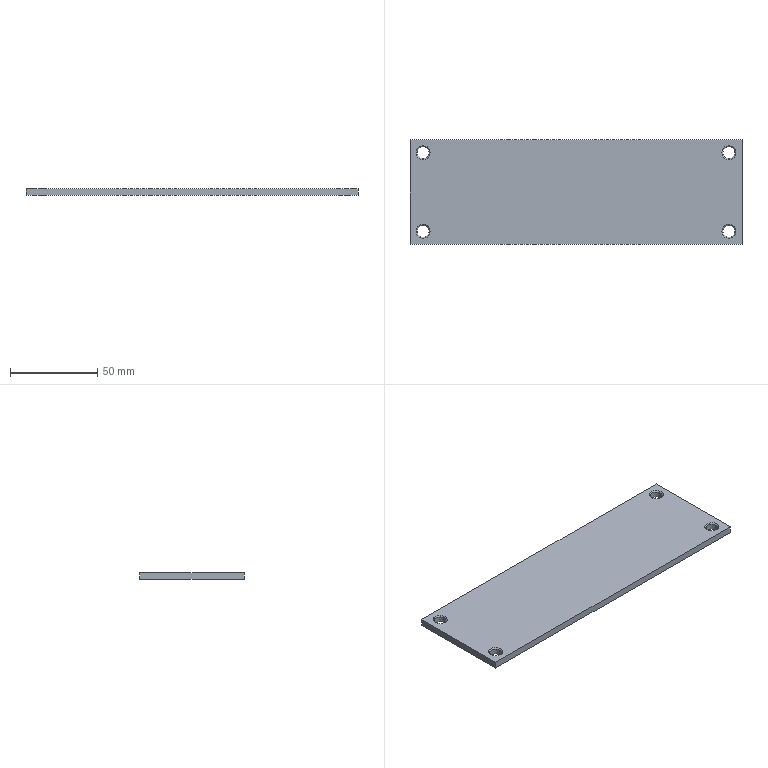Part | STEP file | Plate 2 | 1 solid | 22 faces | box 190 x 60 x 4 mm | volume 45001 mm3 | cone 8 | cylinder 8 | plane 6 | commonest cylinder face diameters 6.8 x8
STEP:
#1=CARTESIAN_POINT('',(-90.9,22.5,3.375));
#2=VERTEX_POINT('',#1);
#3=CARTESIAN_POINT('',(-84.1,22.5,3.375));
#4=VERTEX_POINT('',#3);
#5=CARTESIAN_POINT('',(-87.5,22.5,3.375));
#6=DIRECTION('',(0.,0.,1.));
#7=DIRECTION('',(1.,0.,0.));
#8=AXIS2_PLACEMENT_3D('',#5,#6,#7);
#9=CIRCLE('',#8,3.4);
#10=EDGE_CURVE('',#2,#4,#9,.T.);
#11=ORIENTED_EDGE('',*,*,#10,.F.);
#12=CARTESIAN_POINT('',(-91.525,22.5,4.));
#13=VERTEX_POINT('',#12);
#14=CARTESIAN_POINT('',(-91.525,22.5,4.));
#15=DIRECTION('',(-0.7071,0.,0.7071));
#16=VECTOR('',#15,1000.);
#17=LINE('',#14,#16);
#18=EDGE_CURVE('',#2,#13,#17,.T.);
#19=ORIENTED_EDGE('',*,*,#18,.T.);
#20=CARTESIAN_POINT('',(-83.475,22.5,4.));
#21=VERTEX_POINT('',#20);
#22=CARTESIAN_POINT('',(-87.5,22.5,4.));
#23=DIRECTION('',(0.,0.,1.));
#24=DIRECTION('',(1.,0.,0.));
#25=AXIS2_PLACEMENT_3D('',#22,#23,#24);
#26=CIRCLE('',#25,4.025);
#27=EDGE_CURVE('',#13,#21,#26,.T.);
#28=ORIENTED_EDGE('',*,*,#27,.T.);
#29=CARTESIAN_POINT('',(-83.475,22.5,4.));
#30=DIRECTION('',(0.7071,0.,0.7071));
#31=VECTOR('',#30,1000.);
#32=LINE('',#29,#31);
#33=EDGE_CURVE('',#4,#21,#32,.T.);
#34=ORIENTED_EDGE('',*,*,#33,.F.);
#35=EDGE_LOOP('',(#11,#19,#28,#34));
#36=FACE_OUTER_BOUND('',#35,.T.);
#37=CARTESIAN_POINT('',(-87.5,22.5,4.));
#38=DIRECTION('',(0.,0.,1.));
#39=DIRECTION('',(1.,0.,0.));
#40=AXIS2_PLACEMENT_3D('',#37,#38,#39);
#41=CONICAL_SURFACE('',#40,4.025,0.7854);
#42=ADVANCED_FACE('',(#36),#41,.F.);
#43=CARTESIAN_POINT('',(-84.1,22.5,0.));
#44=VERTEX_POINT('',#43);
#45=CARTESIAN_POINT('',(-90.9,22.5,0.));
#46=VERTEX_POINT('',#45);
#47=CARTESIAN_POINT('',(-87.5,22.5,0.));
#48=DIRECTION('',(0.,0.,-1.));
#49=DIRECTION('',(-1.,0.,0.));
#50=AXIS2_PLACEMENT_3D('',#47,#48,#49);
#51=CIRCLE('',#50,3.4);
#52=EDGE_CURVE('',#44,#46,#51,.T.);
#53=ORIENTED_EDGE('',*,*,#52,.T.);
#54=CARTESIAN_POINT('',(-90.9,22.5,4.));
#55=DIRECTION('',(0.,0.,1.));
#56=VECTOR('',#55,1000.);
#57=LINE('',#54,#56);
#58=EDGE_CURVE('',#46,#2,#57,.T.);
#59=ORIENTED_EDGE('',*,*,#58,.T.);
#60=ORIENTED_EDGE('',*,*,#10,.T.);
#61=CARTESIAN_POINT('',(-84.1,22.5,4.));
#62=DIRECTION('',(0.,0.,1.));
#63=VECTOR('',#62,1000.);
#64=LINE('',#61,#63);
#65=EDGE_CURVE('',#44,#4,#64,.T.);
#66=ORIENTED_EDGE('',*,*,#65,.F.);
#67=EDGE_LOOP('',(#53,#59,#60,#66));
#68=FACE_OUTER_BOUND('',#67,.T.);
#69=CARTESIAN_POINT('',(-87.5,22.5,4.));
#70=DIRECTION('',(0.,0.,1.));
#71=DIRECTION('',(1.,0.,0.));
#72=AXIS2_PLACEMENT_3D('',#69,#70,#71);
#73=CYLINDRICAL_SURFACE('',#72,3.4);
#74=ADVANCED_FACE('',(#68),#73,.F.);
#75=CARTESIAN_POINT('',(84.1,-22.5,3.375));
#76=VERTEX_POINT('',#75);
#77=CARTESIAN_POINT('',(90.9,-22.5,3.375));
#78=VERTEX_POINT('',#77);
#79=CARTESIAN_POINT('',(87.5,-22.5,3.375));
#80=DIRECTION('',(0.,0.,1.));
#81=DIRECTION('',(1.,0.,0.));
#82=AXIS2_PLACEMENT_3D('',#79,#80,#81);
#83=CIRCLE('',#82,3.4);
#84=EDGE_CURVE('',#76,#78,#83,.T.);
#85=ORIENTED_EDGE('',*,*,#84,.F.);
#86=CARTESIAN_POINT('',(83.475,-22.5,4.));
#87=VERTEX_POINT('',#86);
#88=CARTESIAN_POINT('',(83.475,-22.5,4.));
#89=DIRECTION('',(-0.7071,0.,0.7071));
#90=VECTOR('',#89,1000.);
#91=LINE('',#88,#90);
#92=EDGE_CURVE('',#76,#87,#91,.T.);
#93=ORIENTED_EDGE('',*,*,#92,.T.);
#94=CARTESIAN_POINT('',(91.525,-22.5,4.));
#95=VERTEX_POINT('',#94);
#96=CARTESIAN_POINT('',(87.5,-22.5,4.));
#97=DIRECTION('',(0.,0.,1.));
#98=DIRECTION('',(1.,0.,0.));
#99=AXIS2_PLACEMENT_3D('',#96,#97,#98);
#100=CIRCLE('',#99,4.025);
#101=EDGE_CURVE('',#87,#95,#100,.T.);
#102=ORIENTED_EDGE('',*,*,#101,.T.);
#103=CARTESIAN_POINT('',(91.525,-22.5,4.));
#104=DIRECTION('',(0.7071,0.,0.7071));
#105=VECTOR('',#104,1000.);
#106=LINE('',#103,#105);
#107=EDGE_CURVE('',#78,#95,#106,.T.);
#108=ORIENTED_EDGE('',*,*,#107,.F.);
#109=EDGE_LOOP('',(#85,#93,#102,#108));
#110=FACE_OUTER_BOUND('',#109,.T.);
#111=CARTESIAN_POINT('',(87.5,-22.5,4.));
#112=DIRECTION('',(0.,0.,1.));
#113=DIRECTION('',(1.,0.,0.));
#114=AXIS2_PLACEMENT_3D('',#111,#112,#113);
#115=CONICAL_SURFACE('',#114,4.025,0.7854);
#116=ADVANCED_FACE('',(#110),#115,.F.);
#117=CARTESIAN_POINT('',(90.9,-22.5,0.));
#118=VERTEX_POINT('',#117);
#119=CARTESIAN_POINT('',(84.1,-22.5,0.));
#120=VERTEX_POINT('',#119);
#121=CARTESIAN_POINT('',(87.5,-22.5,0.));
#122=DIRECTION('',(0.,0.,-1.));
#123=DIRECTION('',(-1.,0.,0.));
#124=AXIS2_PLACEMENT_3D('',#121,#122,#123);
#125=CIRCLE('',#124,3.4);
#126=EDGE_CURVE('',#118,#120,#125,.T.);
#127=ORIENTED_EDGE('',*,*,#126,.T.);
#128=CARTESIAN_POINT('',(84.1,-22.5,4.));
#129=DIRECTION('',(0.,0.,1.));
#130=VECTOR('',#129,1000.);
#131=LINE('',#128,#130);
#132=EDGE_CURVE('',#120,#76,#131,.T.);
#133=ORIENTED_EDGE('',*,*,#132,.T.);
#134=ORIENTED_EDGE('',*,*,#84,.T.);
#135=CARTESIAN_POINT('',(90.9,-22.5,4.));
#136=DIRECTION('',(0.,0.,1.));
#137=VECTOR('',#136,1000.);
#138=LINE('',#135,#137);
#139=EDGE_CURVE('',#118,#78,#138,.T.);
#140=ORIENTED_EDGE('',*,*,#139,.F.);
#141=EDGE_LOOP('',(#127,#133,#134,#140));
#142=FACE_OUTER_BOUND('',#141,.T.);
#143=CARTESIAN_POINT('',(87.5,-22.5,4.));
#144=DIRECTION('',(0.,0.,1.));
#145=DIRECTION('',(1.,0.,0.));
#146=AXIS2_PLACEMENT_3D('',#143,#144,#145);
#147=CYLINDRICAL_SURFACE('',#146,3.4);
#148=ADVANCED_FACE('',(#142),#147,.F.);
#149=CARTESIAN_POINT('',(84.1,22.5,3.375));
#150=VERTEX_POINT('',#149);
#151=CARTESIAN_POINT('',(90.9,22.5,3.375));
#152=VERTEX_POINT('',#151);
#153=CARTESIAN_POINT('',(87.5,22.5,3.375));
#154=DIRECTION('',(0.,0.,1.));
#155=DIRECTION('',(1.,0.,0.));
#156=AXIS2_PLACEMENT_3D('',#153,#154,#155);
#157=CIRCLE('',#156,3.4);
#158=EDGE_CURVE('',#150,#152,#157,.T.);
#159=ORIENTED_EDGE('',*,*,#158,.F.);
#160=CARTESIAN_POINT('',(83.475,22.5,4.));
#161=VERTEX_POINT('',#160);
#162=CARTESIAN_POINT('',(83.475,22.5,4.));
#163=DIRECTION('',(-0.7071,0.,0.7071));
#164=VECTOR('',#163,1000.);
#165=LINE('',#162,#164);
#166=EDGE_CURVE('',#150,#161,#165,.T.);
#167=ORIENTED_EDGE('',*,*,#166,.T.);
#168=CARTESIAN_POINT('',(91.525,22.5,4.));
#169=VERTEX_POINT('',#168);
#170=CARTESIAN_POINT('',(87.5,22.5,4.));
#171=DIRECTION('',(0.,0.,1.));
#172=DIRECTION('',(1.,0.,0.));
#173=AXIS2_PLACEMENT_3D('',#170,#171,#172);
#174=CIRCLE('',#173,4.025);
#175=EDGE_CURVE('',#161,#169,#174,.T.);
#176=ORIENTED_EDGE('',*,*,#175,.T.);
#177=CARTESIAN_POINT('',(91.525,22.5,4.));
#178=DIRECTION('',(0.7071,0.,0.7071));
#179=VECTOR('',#178,1000.);
#180=LINE('',#177,#179);
#181=EDGE_CURVE('',#152,#169,#180,.T.);
#182=ORIENTED_EDGE('',*,*,#181,.F.);
#183=EDGE_LOOP('',(#159,#167,#176,#182));
#184=FACE_OUTER_BOUND('',#183,.T.);
#185=CARTESIAN_POINT('',(87.5,22.5,4.));
#186=DIRECTION('',(0.,0.,1.));
#187=DIRECTION('',(1.,0.,0.));
#188=AXIS2_PLACEMENT_3D('',#185,#186,#187);
#189=CONICAL_SURFACE('',#188,4.025,0.7854);
#190=ADVANCED_FACE('',(#184),#189,.F.);
#191=CARTESIAN_POINT('',(90.9,22.5,0.));
#192=VERTEX_POINT('',#191);
#193=CARTESIAN_POINT('',(84.1,22.5,0.));
#194=VERTEX_POINT('',#193);
#195=CARTESIAN_POINT('',(87.5,22.5,0.));
#196=DIRECTION('',(0.,0.,-1.));
#197=DIRECTION('',(-1.,0.,0.));
#198=AXIS2_PLACEMENT_3D('',#195,#196,#197);
#199=CIRCLE('',#198,3.4);
#200=EDGE_CURVE('',#192,#194,#199,.T.);
#201=ORIENTED_EDGE('',*,*,#200,.T.);
#202=CARTESIAN_POINT('',(84.1,22.5,4.));
#203=DIRECTION('',(0.,0.,1.));
#204=VECTOR('',#203,1000.);
#205=LINE('',#202,#204);
#206=EDGE_CURVE('',#194,#150,#205,.T.);
#207=ORIENTED_EDGE('',*,*,#206,.T.);
#208=ORIENTED_EDGE('',*,*,#158,.T.);
#209=CARTESIAN_POINT('',(90.9,22.5,4.));
#210=DIRECTION('',(0.,0.,1.));
#211=VECTOR('',#210,1000.);
#212=LINE('',#209,#211);
#213=EDGE_CURVE('',#192,#152,#212,.T.);
#214=ORIENTED_EDGE('',*,*,#213,.F.);
#215=EDGE_LOOP('',(#201,#207,#208,#214));
#216=FACE_OUTER_BOUND('',#215,.T.);
#217=CARTESIAN_POINT('',(87.5,22.5,4.));
#218=DIRECTION('',(0.,0.,1.));
#219=DIRECTION('',(1.,0.,0.));
#220=AXIS2_PLACEMENT_3D('',#217,#218,#219);
#221=CYLINDRICAL_SURFACE('',#220,3.4);
#222=ADVANCED_FACE('',(#216),#221,.F.);
#223=CARTESIAN_POINT('',(-90.9,-22.5,3.375));
#224=VERTEX_POINT('',#223);
#225=CARTESIAN_POINT('',(-84.1,-22.5,3.375));
#226=VERTEX_POINT('',#225);
#227=CARTESIAN_POINT('',(-87.5,-22.5,3.375));
#228=DIRECTION('',(0.,0.,1.));
#229=DIRECTION('',(1.,0.,0.));
#230=AXIS2_PLACEMENT_3D('',#227,#228,#229);
#231=CIRCLE('',#230,3.4);
#232=EDGE_CURVE('',#224,#226,#231,.T.);
#233=ORIENTED_EDGE('',*,*,#232,.F.);
#234=CARTESIAN_POINT('',(-91.525,-22.5,4.));
#235=VERTEX_POINT('',#234);
#236=CARTESIAN_POINT('',(-91.525,-22.5,4.));
#237=DIRECTION('',(-0.7071,0.,0.7071));
#238=VECTOR('',#237,1000.);
#239=LINE('',#236,#238);
#240=EDGE_CURVE('',#224,#235,#239,.T.);
#241=ORIENTED_EDGE('',*,*,#240,.T.);
#242=CARTESIAN_POINT('',(-83.475,-22.5,4.));
#243=VERTEX_POINT('',#242);
#244=CARTESIAN_POINT('',(-87.5,-22.5,4.));
#245=DIRECTION('',(0.,0.,1.));
#246=DIRECTION('',(1.,0.,0.));
#247=AXIS2_PLACEMENT_3D('',#244,#245,#246);
#248=CIRCLE('',#247,4.025);
#249=EDGE_CURVE('',#235,#243,#248,.T.);
#250=ORIENTED_EDGE('',*,*,#249,.T.);
#251=CARTESIAN_POINT('',(-83.475,-22.5,4.));
#252=DIRECTION('',(0.7071,0.,0.7071));
#253=VECTOR('',#252,1000.);
#254=LINE('',#251,#253);
#255=EDGE_CURVE('',#226,#243,#254,.T.);
#256=ORIENTED_EDGE('',*,*,#255,.F.);
#257=EDGE_LOOP('',(#233,#241,#250,#256));
#258=FACE_OUTER_BOUND('',#257,.T.);
#259=CARTESIAN_POINT('',(-87.5,-22.5,4.));
#260=DIRECTION('',(0.,0.,1.));
#261=DIRECTION('',(1.,0.,0.));
#262=AXIS2_PLACEMENT_3D('',#259,#260,#261);
#263=CONICAL_SURFACE('',#262,4.025,0.7854);
#264=ADVANCED_FACE('',(#258),#263,.F.);
#265=CARTESIAN_POINT('',(-84.1,-22.5,0.));
#266=VERTEX_POINT('',#265);
#267=CARTESIAN_POINT('',(-90.9,-22.5,0.));
#268=VERTEX_POINT('',#267);
#269=CARTESIAN_POINT('',(-87.5,-22.5,0.));
#270=DIRECTION('',(0.,0.,-1.));
#271=DIRECTION('',(-1.,0.,0.));
#272=AXIS2_PLACEMENT_3D('',#269,#270,#271);
#273=CIRCLE('',#272,3.4);
#274=EDGE_CURVE('',#266,#268,#273,.T.);
#275=ORIENTED_EDGE('',*,*,#274,.T.);
#276=CARTESIAN_POINT('',(-90.9,-22.5,4.));
#277=DIRECTION('',(0.,0.,1.));
#278=VECTOR('',#277,1000.);
#279=LINE('',#276,#278);
#280=EDGE_CURVE('',#268,#224,#279,.T.);
#281=ORIENTED_EDGE('',*,*,#280,.T.);
#282=ORIENTED_EDGE('',*,*,#232,.T.);
#283=CARTESIAN_POINT('',(-84.1,-22.5,4.));
#284=DIRECTION('',(0.,0.,1.));
#285=VECTOR('',#284,1000.);
#286=LINE('',#283,#285);
#287=EDGE_CURVE('',#266,#226,#286,.T.);
#288=ORIENTED_EDGE('',*,*,#287,.F.);
#289=EDGE_LOOP('',(#275,#281,#282,#288));
#290=FACE_OUTER_BOUND('',#289,.T.);
#291=CARTESIAN_POINT('',(-87.5,-22.5,4.));
#292=DIRECTION('',(0.,0.,1.));
#293=DIRECTION('',(1.,0.,0.));
#294=AXIS2_PLACEMENT_3D('',#291,#292,#293);
#295=CYLINDRICAL_SURFACE('',#294,3.4);
#296=ADVANCED_FACE('',(#290),#295,.F.);
#297=CARTESIAN_POINT('',(95.,30.,4.));
#298=VERTEX_POINT('',#297);
#299=CARTESIAN_POINT('',(-95.,30.,4.));
#300=VERTEX_POINT('',#299);
#301=CARTESIAN_POINT('',(-95.,30.,4.));
#302=DIRECTION('',(-1.,0.,0.));
#303=VECTOR('',#302,1000.);
#304=LINE('',#301,#303);
#305=EDGE_CURVE('',#298,#300,#304,.T.);
#306=ORIENTED_EDGE('',*,*,#305,.T.);
#307=CARTESIAN_POINT('',(-95.,-30.,4.));
#308=VERTEX_POINT('',#307);
#309=CARTESIAN_POINT('',(-95.,30.001,4.));
#310=DIRECTION('',(0.,-1.,0.));
#311=VECTOR('',#310,1000.);
#312=LINE('',#309,#311);
#313=EDGE_CURVE('',#300,#308,#312,.T.);
#314=ORIENTED_EDGE('',*,*,#313,.T.);
#315=CARTESIAN_POINT('',(95.,-30.,4.));
#316=VERTEX_POINT('',#315);
#317=CARTESIAN_POINT('',(-95.,-30.,4.));
#318=DIRECTION('',(1.,0.,0.));
#319=VECTOR('',#318,1000.);
#320=LINE('',#317,#319);
#321=EDGE_CURVE('',#308,#316,#320,.T.);
#322=ORIENTED_EDGE('',*,*,#321,.T.);
#323=CARTESIAN_POINT('',(95.,-30.,4.));
#324=DIRECTION('',(0.,1.,0.));
#325=VECTOR('',#324,1000.);
#326=LINE('',#323,#325);
#327=EDGE_CURVE('',#316,#298,#326,.T.);
#328=ORIENTED_EDGE('',*,*,#327,.T.);
#329=EDGE_LOOP('',(#306,#314,#322,#328));
#330=FACE_OUTER_BOUND('',#329,.T.);
#331=CARTESIAN_POINT('',(-87.5,-22.5,4.));
#332=DIRECTION('',(0.,0.,1.));
#333=DIRECTION('',(1.,0.,0.));
#334=AXIS2_PLACEMENT_3D('',#331,#332,#333);
#335=CIRCLE('',#334,4.025);
#336=EDGE_CURVE('',#243,#235,#335,.T.);
#337=ORIENTED_EDGE('',*,*,#336,.F.);
#338=ORIENTED_EDGE('',*,*,#249,.F.);
#339=EDGE_LOOP('',(#337,#338));
#340=FACE_BOUND('',#339,.T.);
#341=CARTESIAN_POINT('',(87.5,22.5,4.));
#342=DIRECTION('',(0.,0.,1.));
#343=DIRECTION('',(1.,0.,0.));
#344=AXIS2_PLACEMENT_3D('',#341,#342,#343);
#345=CIRCLE('',#344,4.025);
#346=EDGE_CURVE('',#169,#161,#345,.T.);
#347=ORIENTED_EDGE('',*,*,#346,.F.);
#348=ORIENTED_EDGE('',*,*,#175,.F.);
#349=EDGE_LOOP('',(#347,#348));
#350=FACE_BOUND('',#349,.T.);
#351=CARTESIAN_POINT('',(87.5,-22.5,4.));
#352=DIRECTION('',(0.,0.,1.));
#353=DIRECTION('',(1.,0.,0.));
#354=AXIS2_PLACEMENT_3D('',#351,#352,#353);
#355=CIRCLE('',#354,4.025);
#356=EDGE_CURVE('',#95,#87,#355,.T.);
#357=ORIENTED_EDGE('',*,*,#356,.F.);
#358=ORIENTED_EDGE('',*,*,#101,.F.);
#359=EDGE_LOOP('',(#357,#358));
#360=FACE_BOUND('',#359,.T.);
#361=CARTESIAN_POINT('',(-87.5,22.5,4.));
#362=DIRECTION('',(0.,0.,1.));
#363=DIRECTION('',(1.,0.,0.));
#364=AXIS2_PLACEMENT_3D('',#361,#362,#363);
#365=CIRCLE('',#364,4.025);
#366=EDGE_CURVE('',#21,#13,#365,.T.);
#367=ORIENTED_EDGE('',*,*,#366,.F.);
#368=ORIENTED_EDGE('',*,*,#27,.F.);
#369=EDGE_LOOP('',(#367,#368));
#370=FACE_BOUND('',#369,.T.);
#371=CARTESIAN_POINT('',(0.,0.,4.));
#372=DIRECTION('',(0.,0.,-1.));
#373=DIRECTION('',(-1.,0.,0.));
#374=AXIS2_PLACEMENT_3D('',#371,#372,#373);
#375=PLANE('',#374);
#376=ADVANCED_FACE('',(#330,#340,#350,#360,#370),#375,.F.);
#377=CARTESIAN_POINT('',(95.,-30.,0.));
#378=VERTEX_POINT('',#377);
#379=CARTESIAN_POINT('',(95.,30.,0.));
#380=VERTEX_POINT('',#379);
#381=CARTESIAN_POINT('',(95.,-30.,0.));
#382=DIRECTION('',(0.,1.,0.));
#383=VECTOR('',#382,1000.);
#384=LINE('',#381,#383);
#385=EDGE_CURVE('',#378,#380,#384,.T.);
#386=ORIENTED_EDGE('',*,*,#385,.T.);
#387=CARTESIAN_POINT('',(95.,30.,4.));
#388=DIRECTION('',(0.,0.,-1.));
#389=VECTOR('',#388,1000.);
#390=LINE('',#387,#389);
#391=EDGE_CURVE('',#298,#380,#390,.T.);
#392=ORIENTED_EDGE('',*,*,#391,.F.);
#393=ORIENTED_EDGE('',*,*,#327,.F.);
#394=CARTESIAN_POINT('',(95.,-30.,4.));
#395=DIRECTION('',(0.,0.,-1.));
#396=VECTOR('',#395,1000.);
#397=LINE('',#394,#396);
#398=EDGE_CURVE('',#316,#378,#397,.T.);
#399=ORIENTED_EDGE('',*,*,#398,.T.);
#400=EDGE_LOOP('',(#386,#392,#393,#399));
#401=FACE_OUTER_BOUND('',#400,.T.);
#402=CARTESIAN_POINT('',(95.,-30.,4.));
#403=DIRECTION('',(-1.,0.,0.));
#404=DIRECTION('',(0.,0.,1.));
#405=AXIS2_PLACEMENT_3D('',#402,#403,#404);
#406=PLANE('',#405);
#407=ADVANCED_FACE('',(#401),#406,.F.);
#408=CARTESIAN_POINT('',(-95.,30.,0.));
#409=VERTEX_POINT('',#408);
#410=CARTESIAN_POINT('',(-95.,30.,4.));
#411=DIRECTION('',(0.,0.,-1.));
#412=VECTOR('',#411,1000.);
#413=LINE('',#410,#412);
#414=EDGE_CURVE('',#300,#409,#413,.T.);
#415=ORIENTED_EDGE('',*,*,#414,.F.);
#416=ORIENTED_EDGE('',*,*,#305,.F.);
#417=ORIENTED_EDGE('',*,*,#391,.T.);
#418=CARTESIAN_POINT('',(-95.,30.,0.));
#419=DIRECTION('',(-1.,0.,0.));
#420=VECTOR('',#419,1000.);
#421=LINE('',#418,#420);
#422=EDGE_CURVE('',#380,#409,#421,.T.);
#423=ORIENTED_EDGE('',*,*,#422,.T.);
#424=EDGE_LOOP('',(#415,#416,#417,#423));
#425=FACE_OUTER_BOUND('',#424,.T.);
#426=CARTESIAN_POINT('',(-95.,30.,4.));
#427=DIRECTION('',(0.,-1.,0.));
#428=DIRECTION('',(0.,0.,-1.));
#429=AXIS2_PLACEMENT_3D('',#426,#427,#428);
#430=PLANE('',#429);
#431=ADVANCED_FACE('',(#425),#430,.F.);
#432=CARTESIAN_POINT('',(-95.,-30.,0.));
#433=VERTEX_POINT('',#432);
#434=CARTESIAN_POINT('',(-95.,-30.,4.));
#435=DIRECTION('',(0.,0.,-1.));
#436=VECTOR('',#435,1000.);
#437=LINE('',#434,#436);
#438=EDGE_CURVE('',#308,#433,#437,.T.);
#439=ORIENTED_EDGE('',*,*,#438,.F.);
#440=ORIENTED_EDGE('',*,*,#313,.F.);
#441=ORIENTED_EDGE('',*,*,#414,.T.);
#442=CARTESIAN_POINT('',(-95.,-30.,0.));
#443=DIRECTION('',(0.,-1.,0.));
#444=VECTOR('',#443,1000.);
#445=LINE('',#442,#444);
#446=EDGE_CURVE('',#409,#433,#445,.T.);
#447=ORIENTED_EDGE('',*,*,#446,.T.);
#448=EDGE_LOOP('',(#439,#440,#441,#447));
#449=FACE_OUTER_BOUND('',#448,.T.);
#450=CARTESIAN_POINT('',(-95.,-30.,4.));
#451=DIRECTION('',(1.,0.,0.));
#452=DIRECTION('',(0.,0.,-1.));
#453=AXIS2_PLACEMENT_3D('',#450,#451,#452);
#454=PLANE('',#453);
#455=ADVANCED_FACE('',(#449),#454,.F.);
#456=ORIENTED_EDGE('',*,*,#321,.F.);
#457=ORIENTED_EDGE('',*,*,#438,.T.);
#458=CARTESIAN_POINT('',(-95.,-30.,0.));
#459=DIRECTION('',(1.,0.,0.));
#460=VECTOR('',#459,1000.);
#461=LINE('',#458,#460);
#462=EDGE_CURVE('',#433,#378,#461,.T.);
#463=ORIENTED_EDGE('',*,*,#462,.T.);
#464=ORIENTED_EDGE('',*,*,#398,.F.);
#465=EDGE_LOOP('',(#456,#457,#463,#464));
#466=FACE_OUTER_BOUND('',#465,.T.);
#467=CARTESIAN_POINT('',(-95.,-30.,4.));
#468=DIRECTION('',(0.,1.,0.));
#469=DIRECTION('',(0.,0.,1.));
#470=AXIS2_PLACEMENT_3D('',#467,#468,#469);
#471=PLANE('',#470);
#472=ADVANCED_FACE('',(#466),#471,.F.);
#473=ORIENTED_EDGE('',*,*,#52,.F.);
#474=CARTESIAN_POINT('',(-87.5,22.5,0.));
#475=DIRECTION('',(0.,0.,-1.));
#476=DIRECTION('',(-1.,0.,0.));
#477=AXIS2_PLACEMENT_3D('',#474,#475,#476);
#478=CIRCLE('',#477,3.4);
#479=EDGE_CURVE('',#46,#44,#478,.T.);
#480=ORIENTED_EDGE('',*,*,#479,.F.);
#481=EDGE_LOOP('',(#473,#480));
#482=FACE_BOUND('',#481,.T.);
#483=ORIENTED_EDGE('',*,*,#126,.F.);
#484=CARTESIAN_POINT('',(87.5,-22.5,0.));
#485=DIRECTION('',(0.,0.,-1.));
#486=DIRECTION('',(-1.,0.,0.));
#487=AXIS2_PLACEMENT_3D('',#484,#485,#486);
#488=CIRCLE('',#487,3.4);
#489=EDGE_CURVE('',#120,#118,#488,.T.);
#490=ORIENTED_EDGE('',*,*,#489,.F.);
#491=EDGE_LOOP('',(#483,#490));
#492=FACE_BOUND('',#491,.T.);
#493=ORIENTED_EDGE('',*,*,#200,.F.);
#494=CARTESIAN_POINT('',(87.5,22.5,0.));
#495=DIRECTION('',(0.,0.,-1.));
#496=DIRECTION('',(-1.,0.,0.));
#497=AXIS2_PLACEMENT_3D('',#494,#495,#496);
#498=CIRCLE('',#497,3.4);
#499=EDGE_CURVE('',#194,#192,#498,.T.);
#500=ORIENTED_EDGE('',*,*,#499,.F.);
#501=EDGE_LOOP('',(#493,#500));
#502=FACE_BOUND('',#501,.T.);
#503=ORIENTED_EDGE('',*,*,#274,.F.);
#504=CARTESIAN_POINT('',(-87.5,-22.5,0.));
#505=DIRECTION('',(0.,0.,-1.));
#506=DIRECTION('',(-1.,0.,0.));
#507=AXIS2_PLACEMENT_3D('',#504,#505,#506);
#508=CIRCLE('',#507,3.4);
#509=EDGE_CURVE('',#268,#266,#508,.T.);
#510=ORIENTED_EDGE('',*,*,#509,.F.);
#511=EDGE_LOOP('',(#503,#510));
#512=FACE_BOUND('',#511,.T.);
#513=ORIENTED_EDGE('',*,*,#385,.F.);
#514=ORIENTED_EDGE('',*,*,#462,.F.);
#515=ORIENTED_EDGE('',*,*,#446,.F.);
#516=ORIENTED_EDGE('',*,*,#422,.F.);
#517=EDGE_LOOP('',(#513,#514,#515,#516));
#518=FACE_OUTER_BOUND('',#517,.T.);
#519=CARTESIAN_POINT('',(0.,0.,0.));
#520=DIRECTION('',(0.,0.,-1.));
#521=DIRECTION('',(-1.,0.,0.));
#522=AXIS2_PLACEMENT_3D('',#519,#520,#521);
#523=PLANE('',#522);
#524=ADVANCED_FACE('',(#482,#492,#502,#512,#518),#523,.T.);
#525=ORIENTED_EDGE('',*,*,#280,.F.);
#526=ORIENTED_EDGE('',*,*,#509,.T.);
#527=ORIENTED_EDGE('',*,*,#287,.T.);
#528=CARTESIAN_POINT('',(-87.5,-22.5,3.375));
#529=DIRECTION('',(0.,0.,1.));
#530=DIRECTION('',(1.,0.,0.));
#531=AXIS2_PLACEMENT_3D('',#528,#529,#530);
#532=CIRCLE('',#531,3.4);
#533=EDGE_CURVE('',#226,#224,#532,.T.);
#534=ORIENTED_EDGE('',*,*,#533,.T.);
#535=EDGE_LOOP('',(#525,#526,#527,#534));
#536=FACE_OUTER_BOUND('',#535,.T.);
#537=CARTESIAN_POINT('',(-87.5,-22.5,4.));
#538=DIRECTION('',(0.,0.,1.));
#539=DIRECTION('',(1.,0.,0.));
#540=AXIS2_PLACEMENT_3D('',#537,#538,#539);
#541=CYLINDRICAL_SURFACE('',#540,3.4);
#542=ADVANCED_FACE('',(#536),#541,.F.);
#543=ORIENTED_EDGE('',*,*,#240,.F.);
#544=ORIENTED_EDGE('',*,*,#533,.F.);
#545=ORIENTED_EDGE('',*,*,#255,.T.);
#546=ORIENTED_EDGE('',*,*,#336,.T.);
#547=EDGE_LOOP('',(#543,#544,#545,#546));
#548=FACE_OUTER_BOUND('',#547,.T.);
#549=CARTESIAN_POINT('',(-87.5,-22.5,4.));
#550=DIRECTION('',(0.,0.,1.));
#551=DIRECTION('',(1.,0.,0.));
#552=AXIS2_PLACEMENT_3D('',#549,#550,#551);
#553=CONICAL_SURFACE('',#552,4.025,0.7854);
#554=ADVANCED_FACE('',(#548),#553,.F.);
#555=ORIENTED_EDGE('',*,*,#206,.F.);
#556=ORIENTED_EDGE('',*,*,#499,.T.);
#557=ORIENTED_EDGE('',*,*,#213,.T.);
#558=CARTESIAN_POINT('',(87.5,22.5,3.375));
#559=DIRECTION('',(0.,0.,1.));
#560=DIRECTION('',(1.,0.,0.));
#561=AXIS2_PLACEMENT_3D('',#558,#559,#560);
#562=CIRCLE('',#561,3.4);
#563=EDGE_CURVE('',#152,#150,#562,.T.);
#564=ORIENTED_EDGE('',*,*,#563,.T.);
#565=EDGE_LOOP('',(#555,#556,#557,#564));
#566=FACE_OUTER_BOUND('',#565,.T.);
#567=CARTESIAN_POINT('',(87.5,22.5,4.));
#568=DIRECTION('',(0.,0.,1.));
#569=DIRECTION('',(1.,0.,0.));
#570=AXIS2_PLACEMENT_3D('',#567,#568,#569);
#571=CYLINDRICAL_SURFACE('',#570,3.4);
#572=ADVANCED_FACE('',(#566),#571,.F.);
#573=ORIENTED_EDGE('',*,*,#166,.F.);
#574=ORIENTED_EDGE('',*,*,#563,.F.);
#575=ORIENTED_EDGE('',*,*,#181,.T.);
#576=ORIENTED_EDGE('',*,*,#346,.T.);
#577=EDGE_LOOP('',(#573,#574,#575,#576));
#578=FACE_OUTER_BOUND('',#577,.T.);
#579=CARTESIAN_POINT('',(87.5,22.5,4.));
#580=DIRECTION('',(0.,0.,1.));
#581=DIRECTION('',(1.,0.,0.));
#582=AXIS2_PLACEMENT_3D('',#579,#580,#581);
#583=CONICAL_SURFACE('',#582,4.025,0.7854);
#584=ADVANCED_FACE('',(#578),#583,.F.);
#585=ORIENTED_EDGE('',*,*,#132,.F.);
#586=ORIENTED_EDGE('',*,*,#489,.T.);
#587=ORIENTED_EDGE('',*,*,#139,.T.);
#588=CARTESIAN_POINT('',(87.5,-22.5,3.375));
#589=DIRECTION('',(0.,0.,1.));
#590=DIRECTION('',(1.,0.,0.));
#591=AXIS2_PLACEMENT_3D('',#588,#589,#590);
#592=CIRCLE('',#591,3.4);
#593=EDGE_CURVE('',#78,#76,#592,.T.);
#594=ORIENTED_EDGE('',*,*,#593,.T.);
#595=EDGE_LOOP('',(#585,#586,#587,#594));
#596=FACE_OUTER_BOUND('',#595,.T.);
#597=CARTESIAN_POINT('',(87.5,-22.5,4.));
#598=DIRECTION('',(0.,0.,1.));
#599=DIRECTION('',(1.,0.,0.));
#600=AXIS2_PLACEMENT_3D('',#597,#598,#599);
#601=CYLINDRICAL_SURFACE('',#600,3.4);
#602=ADVANCED_FACE('',(#596),#601,.F.);
#603=ORIENTED_EDGE('',*,*,#92,.F.);
#604=ORIENTED_EDGE('',*,*,#593,.F.);
#605=ORIENTED_EDGE('',*,*,#107,.T.);
#606=ORIENTED_EDGE('',*,*,#356,.T.);
#607=EDGE_LOOP('',(#603,#604,#605,#606));
#608=FACE_OUTER_BOUND('',#607,.T.);
#609=CARTESIAN_POINT('',(87.5,-22.5,4.));
#610=DIRECTION('',(0.,0.,1.));
#611=DIRECTION('',(1.,0.,0.));
#612=AXIS2_PLACEMENT_3D('',#609,#610,#611);
#613=CONICAL_SURFACE('',#612,4.025,0.7854);
#614=ADVANCED_FACE('',(#608),#613,.F.);
#615=ORIENTED_EDGE('',*,*,#58,.F.);
#616=ORIENTED_EDGE('',*,*,#479,.T.);
#617=ORIENTED_EDGE('',*,*,#65,.T.);
#618=CARTESIAN_POINT('',(-87.5,22.5,3.375));
#619=DIRECTION('',(0.,0.,1.));
#620=DIRECTION('',(1.,0.,0.));
#621=AXIS2_PLACEMENT_3D('',#618,#619,#620);
#622=CIRCLE('',#621,3.4);
#623=EDGE_CURVE('',#4,#2,#622,.T.);
#624=ORIENTED_EDGE('',*,*,#623,.T.);
#625=EDGE_LOOP('',(#615,#616,#617,#624));
#626=FACE_OUTER_BOUND('',#625,.T.);
#627=CARTESIAN_POINT('',(-87.5,22.5,4.));
#628=DIRECTION('',(0.,0.,1.));
#629=DIRECTION('',(1.,0.,0.));
#630=AXIS2_PLACEMENT_3D('',#627,#628,#629);
#631=CYLINDRICAL_SURFACE('',#630,3.4);
#632=ADVANCED_FACE('',(#626),#631,.F.);
#633=ORIENTED_EDGE('',*,*,#18,.F.);
#634=ORIENTED_EDGE('',*,*,#623,.F.);
#635=ORIENTED_EDGE('',*,*,#33,.T.);
#636=ORIENTED_EDGE('',*,*,#366,.T.);
#637=EDGE_LOOP('',(#633,#634,#635,#636));
#638=FACE_OUTER_BOUND('',#637,.T.);
#639=CARTESIAN_POINT('',(-87.5,22.5,4.));
#640=DIRECTION('',(0.,0.,1.));
#641=DIRECTION('',(1.,0.,0.));
#642=AXIS2_PLACEMENT_3D('',#639,#640,#641);
#643=CONICAL_SURFACE('',#642,4.025,0.7854);
#644=ADVANCED_FACE('',(#638),#643,.F.);
#645=CLOSED_SHELL('',(#42,#74,#116,#148,#190,#222,#264,#296,#376,#407,#431,#455,#472,#524,#542,#554,#572,#584,#602,#614,#632,#644));
#646=MANIFOLD_SOLID_BREP('',#645);
#647=CARTESIAN_POINT('',(0.,0.,0.));
#648=DIRECTION('',(0.,0.,1.));
#649=DIRECTION('',(1.,0.,0.));
#650=AXIS2_PLACEMENT_3D('',#647,#648,#649);
#651=(LENGTH_UNIT()NAMED_UNIT(*)SI_UNIT(.MILLI.,.METRE.));
#652=UNCERTAINTY_MEASURE_WITH_UNIT(LENGTH_MEASURE(0.00001),#651,'','');
#653=(NAMED_UNIT(*)PLANE_ANGLE_UNIT()SI_UNIT($,.RADIAN.));
#654=(NAMED_UNIT(*)SI_UNIT($,.STERADIAN.)SOLID_ANGLE_UNIT());
#655=(GEOMETRIC_REPRESENTATION_CONTEXT(3)GLOBAL_UNCERTAINTY_ASSIGNED_CONTEXT((#652))GLOBAL_UNIT_ASSIGNED_CONTEXT((#651,#653,#654))REPRESENTATION_CONTEXT('',''));
#656=ADVANCED_BREP_SHAPE_REPRESENTATION('',(#646,#650),#655);